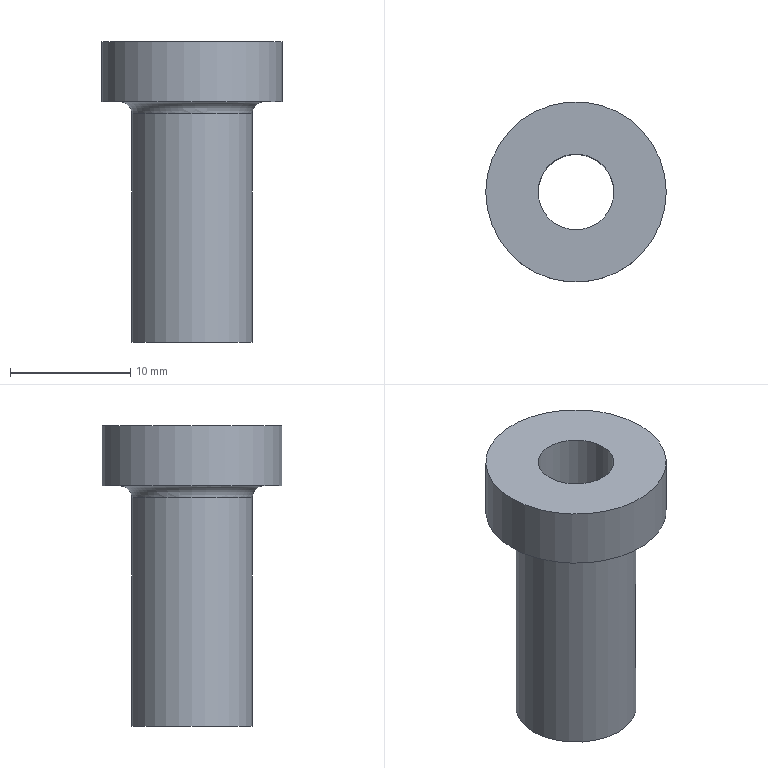Part | NX | features PG_666 2 | 1 solid | 7 faces | box 15 x 15 x 25 mm | volume 1682 mm3 | plane 3 | cylinder 3 | torus 1 | commonest cylinder face diameters 6.3 x1 10 x1 15 x1
STEP:
#1=CARTESIAN_POINT('',(2932.921,-779.947,823.716));
#2=VERTEX_POINT('',#1);
#3=CARTESIAN_POINT('',(2929.771,-779.947,823.716));
#4=DIRECTION('',(0.,0.,-1.));
#5=DIRECTION('',(1.,0.,0.));
#6=AXIS2_PLACEMENT_3D('',#3,#4,#5);
#7=CIRCLE('',#6,3.15);
#8=EDGE_CURVE('',#2,#2,#7,.T.);
#9=ORIENTED_EDGE('',*,*,#8,.F.);
#10=EDGE_LOOP('',(#9));
#11=FACE_BOUND('',#10,.T.);
#12=CARTESIAN_POINT('',(2934.771,-779.947,823.716));
#13=VERTEX_POINT('',#12);
#14=CARTESIAN_POINT('',(2929.771,-779.947,823.716));
#15=DIRECTION('',(0.,0.,-1.));
#16=DIRECTION('',(1.,0.,0.));
#17=AXIS2_PLACEMENT_3D('',#14,#15,#16);
#18=CIRCLE('',#17,5.);
#19=EDGE_CURVE('',#13,#13,#18,.T.);
#20=ORIENTED_EDGE('',*,*,#19,.T.);
#21=EDGE_LOOP('',(#20));
#22=FACE_BOUND('',#21,.T.);
#23=CARTESIAN_POINT('',(2929.771,-779.947,823.716));
#24=DIRECTION('',(0.,0.,-1.));
#25=DIRECTION('',(-1.,0.,0.));
#26=AXIS2_PLACEMENT_3D('',#23,#24,#25);
#27=PLANE('',#26);
#28=ADVANCED_FACE('',(#11,#22),#27,.T.);
#29=CARTESIAN_POINT('',(2924.771,-779.947,842.716));
#30=VERTEX_POINT('',#29);
#31=CARTESIAN_POINT('',(2929.771,-779.947,842.716));
#32=DIRECTION('',(0.,0.,1.));
#33=DIRECTION('',(-1.,0.,0.));
#34=AXIS2_PLACEMENT_3D('',#31,#32,#33);
#35=CIRCLE('',#34,5.);
#36=EDGE_CURVE('',#30,#30,#35,.T.);
#37=ORIENTED_EDGE('',*,*,#36,.F.);
#38=EDGE_LOOP('',(#37));
#39=FACE_BOUND('',#38,.T.);
#40=ORIENTED_EDGE('',*,*,#19,.F.);
#41=EDGE_LOOP('',(#40));
#42=FACE_BOUND('',#41,.T.);
#43=CARTESIAN_POINT('',(2929.771,-779.947,808.716));
#44=DIRECTION('',(0.,0.,1.));
#45=DIRECTION('',(1.,0.,0.));
#46=AXIS2_PLACEMENT_3D('',#43,#44,#45);
#47=CYLINDRICAL_SURFACE('',#46,5.);
#48=ADVANCED_FACE('',(#39,#42),#47,.T.);
#49=CARTESIAN_POINT('',(2932.921,-779.947,848.716));
#50=VERTEX_POINT('',#49);
#51=CARTESIAN_POINT('',(2929.771,-779.947,848.716));
#52=DIRECTION('',(0.,0.,-1.));
#53=DIRECTION('',(1.,0.,0.));
#54=AXIS2_PLACEMENT_3D('',#51,#52,#53);
#55=CIRCLE('',#54,3.15);
#56=EDGE_CURVE('',#50,#50,#55,.F.);
#57=ORIENTED_EDGE('',*,*,#56,.F.);
#58=EDGE_LOOP('',(#57));
#59=FACE_BOUND('',#58,.T.);
#60=CARTESIAN_POINT('',(2937.271,-779.947,848.716));
#61=VERTEX_POINT('',#60);
#62=CARTESIAN_POINT('',(2929.771,-779.947,848.716));
#63=DIRECTION('',(0.,0.,1.));
#64=DIRECTION('',(1.,0.,0.));
#65=AXIS2_PLACEMENT_3D('',#62,#63,#64);
#66=CIRCLE('',#65,7.5);
#67=EDGE_CURVE('',#61,#61,#66,.T.);
#68=ORIENTED_EDGE('',*,*,#67,.T.);
#69=EDGE_LOOP('',(#68));
#70=FACE_BOUND('',#69,.T.);
#71=CARTESIAN_POINT('',(2929.771,-779.947,848.716));
#72=DIRECTION('',(0.,0.,1.));
#73=DIRECTION('',(1.,0.,0.));
#74=AXIS2_PLACEMENT_3D('',#71,#72,#73);
#75=PLANE('',#74);
#76=ADVANCED_FACE('',(#59,#70),#75,.T.);
#77=CARTESIAN_POINT('',(2923.771,-779.947,843.716));
#78=VERTEX_POINT('',#77);
#79=CARTESIAN_POINT('',(2929.771,-779.947,843.716));
#80=DIRECTION('',(0.,0.,1.));
#81=DIRECTION('',(-1.,0.,0.));
#82=AXIS2_PLACEMENT_3D('',#79,#80,#81);
#83=CIRCLE('',#82,6.);
#84=EDGE_CURVE('',#78,#78,#83,.F.);
#85=ORIENTED_EDGE('',*,*,#84,.F.);
#86=EDGE_LOOP('',(#85));
#87=FACE_BOUND('',#86,.T.);
#88=CARTESIAN_POINT('',(2937.271,-779.947,843.716));
#89=VERTEX_POINT('',#88);
#90=CARTESIAN_POINT('',(2929.771,-779.947,843.716));
#91=DIRECTION('',(0.,0.,-1.));
#92=DIRECTION('',(1.,0.,0.));
#93=AXIS2_PLACEMENT_3D('',#90,#91,#92);
#94=CIRCLE('',#93,7.5);
#95=EDGE_CURVE('',#89,#89,#94,.T.);
#96=ORIENTED_EDGE('',*,*,#95,.T.);
#97=EDGE_LOOP('',(#96));
#98=FACE_BOUND('',#97,.T.);
#99=CARTESIAN_POINT('',(2929.771,-779.947,843.716));
#100=DIRECTION('',(0.,0.,-1.));
#101=DIRECTION('',(-1.,0.,0.));
#102=AXIS2_PLACEMENT_3D('',#99,#100,#101);
#103=PLANE('',#102);
#104=ADVANCED_FACE('',(#87,#98),#103,.T.);
#105=ORIENTED_EDGE('',*,*,#67,.F.);
#106=EDGE_LOOP('',(#105));
#107=FACE_BOUND('',#106,.T.);
#108=ORIENTED_EDGE('',*,*,#95,.F.);
#109=EDGE_LOOP('',(#108));
#110=FACE_BOUND('',#109,.T.);
#111=CARTESIAN_POINT('',(2929.771,-779.947,843.716));
#112=DIRECTION('',(0.,0.,1.));
#113=DIRECTION('',(1.,0.,0.));
#114=AXIS2_PLACEMENT_3D('',#111,#112,#113);
#115=CYLINDRICAL_SURFACE('',#114,7.5);
#116=ADVANCED_FACE('',(#107,#110),#115,.T.);
#117=ORIENTED_EDGE('',*,*,#56,.T.);
#118=EDGE_LOOP('',(#117));
#119=FACE_BOUND('',#118,.T.);
#120=ORIENTED_EDGE('',*,*,#8,.T.);
#121=EDGE_LOOP('',(#120));
#122=FACE_BOUND('',#121,.T.);
#123=CARTESIAN_POINT('',(2929.771,-779.947,808.716));
#124=DIRECTION('',(0.,0.,1.));
#125=DIRECTION('',(1.,0.,0.));
#126=AXIS2_PLACEMENT_3D('',#123,#124,#125);
#127=CYLINDRICAL_SURFACE('',#126,3.15);
#128=ADVANCED_FACE('',(#119,#122),#127,.F.);
#129=ORIENTED_EDGE('',*,*,#36,.T.);
#130=EDGE_LOOP('',(#129));
#131=FACE_BOUND('',#130,.T.);
#132=ORIENTED_EDGE('',*,*,#84,.T.);
#133=EDGE_LOOP('',(#132));
#134=FACE_BOUND('',#133,.T.);
#135=CARTESIAN_POINT('',(2929.771,-779.947,842.716));
#136=DIRECTION('',(0.,0.,-1.));
#137=DIRECTION('',(-1.,0.,0.));
#138=AXIS2_PLACEMENT_3D('',#135,#136,#137);
#139=TOROIDAL_SURFACE('',#138,6.,1.);
#140=ADVANCED_FACE('',(#131,#134),#139,.F.);
#141=CLOSED_SHELL('',(#28,#48,#76,#104,#116,#128,#140));
#142=MANIFOLD_SOLID_BREP('',#141);
#143=(LENGTH_UNIT()NAMED_UNIT(*)SI_UNIT(.MILLI.,.METRE.));
#144=UNCERTAINTY_MEASURE_WITH_UNIT(LENGTH_MEASURE(0.00001),#143,'','');
#145=(NAMED_UNIT(*)PLANE_ANGLE_UNIT()SI_UNIT($,.RADIAN.));
#146=(NAMED_UNIT(*)SI_UNIT($,.STERADIAN.)SOLID_ANGLE_UNIT());
#147=(GEOMETRIC_REPRESENTATION_CONTEXT(3)GLOBAL_UNCERTAINTY_ASSIGNED_CONTEXT((#144))GLOBAL_UNIT_ASSIGNED_CONTEXT((#143,#145,#146))REPRESENTATION_CONTEXT('',''));
#148=ADVANCED_BREP_SHAPE_REPRESENTATION('',(#142),#147);